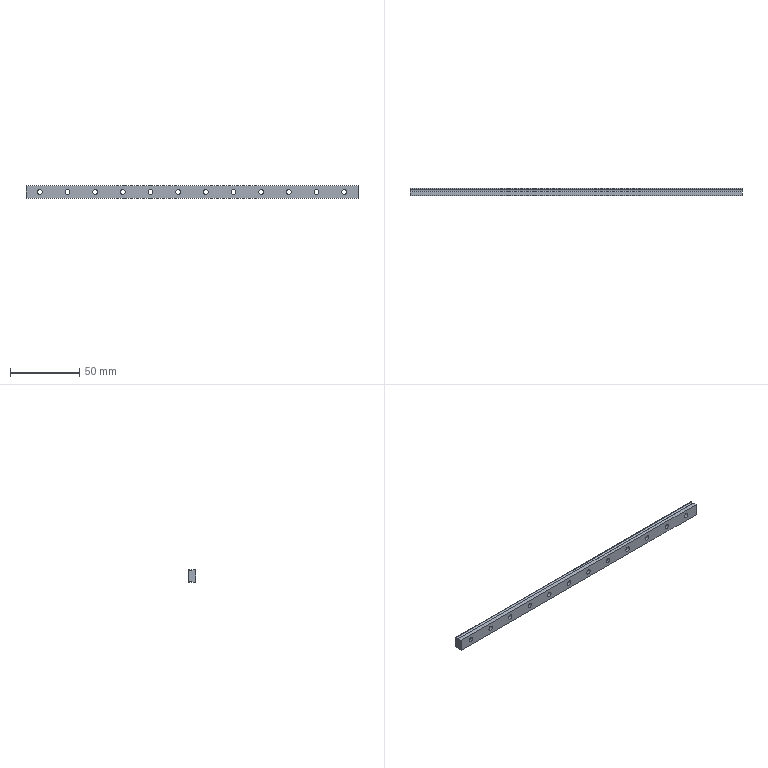Part | STEP file | RSR9KM1-250-1 | 1 solid | 48 faces | box 240 x 5.5 x 9 mm | volume 9857 mm3 | cylinder 26 | plane 22 | commonest cylinder face diameters 3.5 x12 6 x12 2 x2
STEP:
#1=CARTESIAN_POINT('',(230.,0.,4.5));
#2=VERTEX_POINT('',#1);
#3=CARTESIAN_POINT('',(230.,0.,-4.5));
#4=VERTEX_POINT('',#3);
#5=CARTESIAN_POINT('',(230.,0.,4.5));
#6=DIRECTION('',(0.,0.,-1.));
#7=VECTOR('',#6,1000.);
#8=LINE('',#5,#7);
#9=EDGE_CURVE('',#2,#4,#8,.T.);
#10=ORIENTED_EDGE('',*,*,#9,.F.);
#11=CARTESIAN_POINT('',(-10.,0.,4.5));
#12=VERTEX_POINT('',#11);
#13=CARTESIAN_POINT('',(-5.,0.,4.5));
#14=DIRECTION('',(-1.,0.,0.));
#15=VECTOR('',#14,1000.);
#16=LINE('',#13,#15);
#17=EDGE_CURVE('',#2,#12,#16,.T.);
#18=ORIENTED_EDGE('',*,*,#17,.T.);
#19=CARTESIAN_POINT('',(-10.,0.,-4.5));
#20=VERTEX_POINT('',#19);
#21=CARTESIAN_POINT('',(-10.,0.,-4.5));
#22=DIRECTION('',(0.,0.,1.));
#23=VECTOR('',#22,1000.);
#24=LINE('',#21,#23);
#25=EDGE_CURVE('',#20,#12,#24,.T.);
#26=ORIENTED_EDGE('',*,*,#25,.F.);
#27=CARTESIAN_POINT('',(-5.,0.,-4.5));
#28=DIRECTION('',(1.,0.,0.));
#29=VECTOR('',#28,1000.);
#30=LINE('',#27,#29);
#31=EDGE_CURVE('',#20,#4,#30,.T.);
#32=ORIENTED_EDGE('',*,*,#31,.T.);
#33=EDGE_LOOP('',(#10,#18,#26,#32));
#34=FACE_OUTER_BOUND('',#33,.T.);
#35=CARTESIAN_POINT('',(0.,0.,1.75));
#36=VERTEX_POINT('',#35);
#37=CARTESIAN_POINT('',(0.,0.,0.));
#38=DIRECTION('',(0.,1.,0.));
#39=DIRECTION('',(0.,0.,1.));
#40=AXIS2_PLACEMENT_3D('',#37,#38,#39);
#41=CIRCLE('',#40,1.75);
#42=EDGE_CURVE('',#36,#36,#41,.T.);
#43=ORIENTED_EDGE('',*,*,#42,.T.);
#44=EDGE_LOOP('',(#43));
#45=FACE_BOUND('',#44,.T.);
#46=CARTESIAN_POINT('',(220.,0.,1.75));
#47=VERTEX_POINT('',#46);
#48=CARTESIAN_POINT('',(220.,0.,0.));
#49=DIRECTION('',(0.,1.,0.));
#50=DIRECTION('',(0.,0.,1.));
#51=AXIS2_PLACEMENT_3D('',#48,#49,#50);
#52=CIRCLE('',#51,1.75);
#53=EDGE_CURVE('',#47,#47,#52,.T.);
#54=ORIENTED_EDGE('',*,*,#53,.T.);
#55=EDGE_LOOP('',(#54));
#56=FACE_BOUND('',#55,.T.);
#57=CARTESIAN_POINT('',(200.,0.,1.75));
#58=VERTEX_POINT('',#57);
#59=CARTESIAN_POINT('',(200.,0.,0.));
#60=DIRECTION('',(0.,1.,0.));
#61=DIRECTION('',(0.,0.,1.));
#62=AXIS2_PLACEMENT_3D('',#59,#60,#61);
#63=CIRCLE('',#62,1.75);
#64=EDGE_CURVE('',#58,#58,#63,.T.);
#65=ORIENTED_EDGE('',*,*,#64,.T.);
#66=EDGE_LOOP('',(#65));
#67=FACE_BOUND('',#66,.T.);
#68=CARTESIAN_POINT('',(180.,0.,1.75));
#69=VERTEX_POINT('',#68);
#70=CARTESIAN_POINT('',(180.,0.,0.));
#71=DIRECTION('',(0.,1.,0.));
#72=DIRECTION('',(0.,0.,1.));
#73=AXIS2_PLACEMENT_3D('',#70,#71,#72);
#74=CIRCLE('',#73,1.75);
#75=EDGE_CURVE('',#69,#69,#74,.T.);
#76=ORIENTED_EDGE('',*,*,#75,.T.);
#77=EDGE_LOOP('',(#76));
#78=FACE_BOUND('',#77,.T.);
#79=CARTESIAN_POINT('',(160.,0.,1.75));
#80=VERTEX_POINT('',#79);
#81=CARTESIAN_POINT('',(160.,0.,0.));
#82=DIRECTION('',(0.,1.,0.));
#83=DIRECTION('',(0.,0.,1.));
#84=AXIS2_PLACEMENT_3D('',#81,#82,#83);
#85=CIRCLE('',#84,1.75);
#86=EDGE_CURVE('',#80,#80,#85,.T.);
#87=ORIENTED_EDGE('',*,*,#86,.T.);
#88=EDGE_LOOP('',(#87));
#89=FACE_BOUND('',#88,.T.);
#90=CARTESIAN_POINT('',(140.,0.,1.75));
#91=VERTEX_POINT('',#90);
#92=CARTESIAN_POINT('',(140.,0.,0.));
#93=DIRECTION('',(0.,1.,0.));
#94=DIRECTION('',(0.,0.,1.));
#95=AXIS2_PLACEMENT_3D('',#92,#93,#94);
#96=CIRCLE('',#95,1.75);
#97=EDGE_CURVE('',#91,#91,#96,.T.);
#98=ORIENTED_EDGE('',*,*,#97,.T.);
#99=EDGE_LOOP('',(#98));
#100=FACE_BOUND('',#99,.T.);
#101=CARTESIAN_POINT('',(120.,0.,1.75));
#102=VERTEX_POINT('',#101);
#103=CARTESIAN_POINT('',(120.,0.,0.));
#104=DIRECTION('',(0.,1.,0.));
#105=DIRECTION('',(0.,0.,1.));
#106=AXIS2_PLACEMENT_3D('',#103,#104,#105);
#107=CIRCLE('',#106,1.75);
#108=EDGE_CURVE('',#102,#102,#107,.T.);
#109=ORIENTED_EDGE('',*,*,#108,.T.);
#110=EDGE_LOOP('',(#109));
#111=FACE_BOUND('',#110,.T.);
#112=CARTESIAN_POINT('',(100.,0.,1.75));
#113=VERTEX_POINT('',#112);
#114=CARTESIAN_POINT('',(100.,0.,0.));
#115=DIRECTION('',(0.,1.,0.));
#116=DIRECTION('',(0.,0.,1.));
#117=AXIS2_PLACEMENT_3D('',#114,#115,#116);
#118=CIRCLE('',#117,1.75);
#119=EDGE_CURVE('',#113,#113,#118,.T.);
#120=ORIENTED_EDGE('',*,*,#119,.T.);
#121=EDGE_LOOP('',(#120));
#122=FACE_BOUND('',#121,.T.);
#123=CARTESIAN_POINT('',(80.,0.,1.75));
#124=VERTEX_POINT('',#123);
#125=CARTESIAN_POINT('',(80.,0.,0.));
#126=DIRECTION('',(0.,1.,0.));
#127=DIRECTION('',(0.,0.,1.));
#128=AXIS2_PLACEMENT_3D('',#125,#126,#127);
#129=CIRCLE('',#128,1.75);
#130=EDGE_CURVE('',#124,#124,#129,.T.);
#131=ORIENTED_EDGE('',*,*,#130,.T.);
#132=EDGE_LOOP('',(#131));
#133=FACE_BOUND('',#132,.T.);
#134=CARTESIAN_POINT('',(60.,0.,1.75));
#135=VERTEX_POINT('',#134);
#136=CARTESIAN_POINT('',(60.,0.,0.));
#137=DIRECTION('',(0.,1.,0.));
#138=DIRECTION('',(0.,0.,1.));
#139=AXIS2_PLACEMENT_3D('',#136,#137,#138);
#140=CIRCLE('',#139,1.75);
#141=EDGE_CURVE('',#135,#135,#140,.T.);
#142=ORIENTED_EDGE('',*,*,#141,.T.);
#143=EDGE_LOOP('',(#142));
#144=FACE_BOUND('',#143,.T.);
#145=CARTESIAN_POINT('',(40.,0.,1.75));
#146=VERTEX_POINT('',#145);
#147=CARTESIAN_POINT('',(40.,0.,0.));
#148=DIRECTION('',(0.,1.,0.));
#149=DIRECTION('',(0.,0.,1.));
#150=AXIS2_PLACEMENT_3D('',#147,#148,#149);
#151=CIRCLE('',#150,1.75);
#152=EDGE_CURVE('',#146,#146,#151,.T.);
#153=ORIENTED_EDGE('',*,*,#152,.T.);
#154=EDGE_LOOP('',(#153));
#155=FACE_BOUND('',#154,.T.);
#156=CARTESIAN_POINT('',(20.,0.,1.75));
#157=VERTEX_POINT('',#156);
#158=CARTESIAN_POINT('',(20.,0.,0.));
#159=DIRECTION('',(0.,1.,0.));
#160=DIRECTION('',(0.,0.,1.));
#161=AXIS2_PLACEMENT_3D('',#158,#159,#160);
#162=CIRCLE('',#161,1.75);
#163=EDGE_CURVE('',#157,#157,#162,.T.);
#164=ORIENTED_EDGE('',*,*,#163,.T.);
#165=EDGE_LOOP('',(#164));
#166=FACE_BOUND('',#165,.T.);
#167=CARTESIAN_POINT('',(-5.,0.,-4.5));
#168=DIRECTION('',(0.,-1.,0.));
#169=DIRECTION('',(0.,0.,-1.));
#170=AXIS2_PLACEMENT_3D('',#167,#168,#169);
#171=PLANE('',#170);
#172=ADVANCED_FACE('',(#34,#45,#56,#67,#78,#89,#100,#111,#122,#133,#144,#155,#166),#171,.T.);
#173=CARTESIAN_POINT('',(230.,2.811,-4.5));
#174=VERTEX_POINT('',#173);
#175=CARTESIAN_POINT('',(230.,5.5,-4.5));
#176=DIRECTION('',(0.,-1.,0.));
#177=VECTOR('',#176,1000.);
#178=LINE('',#175,#177);
#179=EDGE_CURVE('',#174,#4,#178,.T.);
#180=ORIENTED_EDGE('',*,*,#179,.T.);
#181=ORIENTED_EDGE('',*,*,#31,.F.);
#182=CARTESIAN_POINT('',(-10.,2.811,-4.5));
#183=VERTEX_POINT('',#182);
#184=CARTESIAN_POINT('',(-10.,2.811,-4.5));
#185=DIRECTION('',(0.,-1.,0.));
#186=VECTOR('',#185,1000.);
#187=LINE('',#184,#186);
#188=EDGE_CURVE('',#183,#20,#187,.T.);
#189=ORIENTED_EDGE('',*,*,#188,.F.);
#190=CARTESIAN_POINT('',(-5.,2.811,-4.5));
#191=DIRECTION('',(1.,0.,0.));
#192=VECTOR('',#191,1000.);
#193=LINE('',#190,#192);
#194=EDGE_CURVE('',#183,#174,#193,.T.);
#195=ORIENTED_EDGE('',*,*,#194,.T.);
#196=EDGE_LOOP('',(#180,#181,#189,#195));
#197=FACE_OUTER_BOUND('',#196,.T.);
#198=CARTESIAN_POINT('',(-5.,2.811,-4.5));
#199=DIRECTION('',(0.,0.,-1.));
#200=DIRECTION('',(-1.,0.,0.));
#201=AXIS2_PLACEMENT_3D('',#198,#199,#200);
#202=PLANE('',#201);
#203=ADVANCED_FACE('',(#197),#202,.T.);
#204=CARTESIAN_POINT('',(230.,2.811,4.5));
#205=VERTEX_POINT('',#204);
#206=CARTESIAN_POINT('',(230.,5.5,4.5));
#207=DIRECTION('',(0.,-1.,0.));
#208=VECTOR('',#207,1000.);
#209=LINE('',#206,#208);
#210=EDGE_CURVE('',#205,#2,#209,.T.);
#211=ORIENTED_EDGE('',*,*,#210,.F.);
#212=CARTESIAN_POINT('',(-10.,2.811,4.5));
#213=VERTEX_POINT('',#212);
#214=CARTESIAN_POINT('',(-5.,2.811,4.5));
#215=DIRECTION('',(-1.,0.,0.));
#216=VECTOR('',#215,1000.);
#217=LINE('',#214,#216);
#218=EDGE_CURVE('',#205,#213,#217,.T.);
#219=ORIENTED_EDGE('',*,*,#218,.T.);
#220=CARTESIAN_POINT('',(-10.,0.,4.5));
#221=DIRECTION('',(0.,1.,0.));
#222=VECTOR('',#221,1000.);
#223=LINE('',#220,#222);
#224=EDGE_CURVE('',#12,#213,#223,.T.);
#225=ORIENTED_EDGE('',*,*,#224,.F.);
#226=ORIENTED_EDGE('',*,*,#17,.F.);
#227=EDGE_LOOP('',(#211,#219,#225,#226));
#228=FACE_OUTER_BOUND('',#227,.T.);
#229=CARTESIAN_POINT('',(-5.,0.,4.5));
#230=DIRECTION('',(0.,0.,1.));
#231=DIRECTION('',(1.,0.,0.));
#232=AXIS2_PLACEMENT_3D('',#229,#230,#231);
#233=PLANE('',#232);
#234=ADVANCED_FACE('',(#228),#233,.T.);
#235=ORIENTED_EDGE('',*,*,#42,.F.);
#236=EDGE_LOOP('',(#235));
#237=FACE_OUTER_BOUND('',#236,.T.);
#238=CARTESIAN_POINT('',(0.,2.2,1.75));
#239=VERTEX_POINT('',#238);
#240=CARTESIAN_POINT('',(0.,2.2,0.));
#241=DIRECTION('',(0.,-1.,0.));
#242=DIRECTION('',(0.,0.,1.));
#243=AXIS2_PLACEMENT_3D('',#240,#241,#242);
#244=CIRCLE('',#243,1.75);
#245=EDGE_CURVE('',#239,#239,#244,.T.);
#246=ORIENTED_EDGE('',*,*,#245,.F.);
#247=EDGE_LOOP('',(#246));
#248=FACE_OUTER_BOUND('',#247,.T.);
#249=CARTESIAN_POINT('',(0.,1.1,0.));
#250=DIRECTION('',(0.,1.,0.));
#251=DIRECTION('',(0.,0.,1.));
#252=AXIS2_PLACEMENT_3D('',#249,#250,#251);
#253=CYLINDRICAL_SURFACE('',#252,1.75);
#254=ADVANCED_FACE('',(#237,#248),#253,.F.);
#255=ORIENTED_EDGE('',*,*,#53,.F.);
#256=EDGE_LOOP('',(#255));
#257=FACE_OUTER_BOUND('',#256,.T.);
#258=CARTESIAN_POINT('',(220.,2.2,1.75));
#259=VERTEX_POINT('',#258);
#260=CARTESIAN_POINT('',(220.,2.2,0.));
#261=DIRECTION('',(0.,-1.,0.));
#262=DIRECTION('',(0.,0.,1.));
#263=AXIS2_PLACEMENT_3D('',#260,#261,#262);
#264=CIRCLE('',#263,1.75);
#265=EDGE_CURVE('',#259,#259,#264,.T.);
#266=ORIENTED_EDGE('',*,*,#265,.F.);
#267=EDGE_LOOP('',(#266));
#268=FACE_OUTER_BOUND('',#267,.T.);
#269=CARTESIAN_POINT('',(220.,1.1,0.));
#270=DIRECTION('',(0.,1.,0.));
#271=DIRECTION('',(0.,0.,1.));
#272=AXIS2_PLACEMENT_3D('',#269,#270,#271);
#273=CYLINDRICAL_SURFACE('',#272,1.75);
#274=ADVANCED_FACE('',(#257,#268),#273,.F.);
#275=ORIENTED_EDGE('',*,*,#64,.F.);
#276=EDGE_LOOP('',(#275));
#277=FACE_OUTER_BOUND('',#276,.T.);
#278=CARTESIAN_POINT('',(200.,2.2,1.75));
#279=VERTEX_POINT('',#278);
#280=CARTESIAN_POINT('',(200.,2.2,0.));
#281=DIRECTION('',(0.,-1.,0.));
#282=DIRECTION('',(0.,0.,1.));
#283=AXIS2_PLACEMENT_3D('',#280,#281,#282);
#284=CIRCLE('',#283,1.75);
#285=EDGE_CURVE('',#279,#279,#284,.T.);
#286=ORIENTED_EDGE('',*,*,#285,.F.);
#287=EDGE_LOOP('',(#286));
#288=FACE_OUTER_BOUND('',#287,.T.);
#289=CARTESIAN_POINT('',(200.,1.1,0.));
#290=DIRECTION('',(0.,1.,0.));
#291=DIRECTION('',(0.,0.,1.));
#292=AXIS2_PLACEMENT_3D('',#289,#290,#291);
#293=CYLINDRICAL_SURFACE('',#292,1.75);
#294=ADVANCED_FACE('',(#277,#288),#293,.F.);
#295=ORIENTED_EDGE('',*,*,#75,.F.);
#296=EDGE_LOOP('',(#295));
#297=FACE_OUTER_BOUND('',#296,.T.);
#298=CARTESIAN_POINT('',(180.,2.2,1.75));
#299=VERTEX_POINT('',#298);
#300=CARTESIAN_POINT('',(180.,2.2,0.));
#301=DIRECTION('',(0.,-1.,0.));
#302=DIRECTION('',(0.,0.,1.));
#303=AXIS2_PLACEMENT_3D('',#300,#301,#302);
#304=CIRCLE('',#303,1.75);
#305=EDGE_CURVE('',#299,#299,#304,.T.);
#306=ORIENTED_EDGE('',*,*,#305,.F.);
#307=EDGE_LOOP('',(#306));
#308=FACE_OUTER_BOUND('',#307,.T.);
#309=CARTESIAN_POINT('',(180.,1.1,0.));
#310=DIRECTION('',(0.,1.,0.));
#311=DIRECTION('',(0.,0.,1.));
#312=AXIS2_PLACEMENT_3D('',#309,#310,#311);
#313=CYLINDRICAL_SURFACE('',#312,1.75);
#314=ADVANCED_FACE('',(#297,#308),#313,.F.);
#315=ORIENTED_EDGE('',*,*,#86,.F.);
#316=EDGE_LOOP('',(#315));
#317=FACE_OUTER_BOUND('',#316,.T.);
#318=CARTESIAN_POINT('',(160.,2.2,1.75));
#319=VERTEX_POINT('',#318);
#320=CARTESIAN_POINT('',(160.,2.2,0.));
#321=DIRECTION('',(0.,-1.,0.));
#322=DIRECTION('',(0.,0.,1.));
#323=AXIS2_PLACEMENT_3D('',#320,#321,#322);
#324=CIRCLE('',#323,1.75);
#325=EDGE_CURVE('',#319,#319,#324,.T.);
#326=ORIENTED_EDGE('',*,*,#325,.F.);
#327=EDGE_LOOP('',(#326));
#328=FACE_OUTER_BOUND('',#327,.T.);
#329=CARTESIAN_POINT('',(160.,1.1,0.));
#330=DIRECTION('',(0.,1.,0.));
#331=DIRECTION('',(0.,0.,1.));
#332=AXIS2_PLACEMENT_3D('',#329,#330,#331);
#333=CYLINDRICAL_SURFACE('',#332,1.75);
#334=ADVANCED_FACE('',(#317,#328),#333,.F.);
#335=ORIENTED_EDGE('',*,*,#97,.F.);
#336=EDGE_LOOP('',(#335));
#337=FACE_OUTER_BOUND('',#336,.T.);
#338=CARTESIAN_POINT('',(140.,2.2,1.75));
#339=VERTEX_POINT('',#338);
#340=CARTESIAN_POINT('',(140.,2.2,0.));
#341=DIRECTION('',(0.,-1.,0.));
#342=DIRECTION('',(0.,0.,1.));
#343=AXIS2_PLACEMENT_3D('',#340,#341,#342);
#344=CIRCLE('',#343,1.75);
#345=EDGE_CURVE('',#339,#339,#344,.T.);
#346=ORIENTED_EDGE('',*,*,#345,.F.);
#347=EDGE_LOOP('',(#346));
#348=FACE_OUTER_BOUND('',#347,.T.);
#349=CARTESIAN_POINT('',(140.,1.1,0.));
#350=DIRECTION('',(0.,1.,0.));
#351=DIRECTION('',(0.,0.,1.));
#352=AXIS2_PLACEMENT_3D('',#349,#350,#351);
#353=CYLINDRICAL_SURFACE('',#352,1.75);
#354=ADVANCED_FACE('',(#337,#348),#353,.F.);
#355=ORIENTED_EDGE('',*,*,#108,.F.);
#356=EDGE_LOOP('',(#355));
#357=FACE_OUTER_BOUND('',#356,.T.);
#358=CARTESIAN_POINT('',(120.,2.2,1.75));
#359=VERTEX_POINT('',#358);
#360=CARTESIAN_POINT('',(120.,2.2,0.));
#361=DIRECTION('',(0.,-1.,0.));
#362=DIRECTION('',(0.,0.,1.));
#363=AXIS2_PLACEMENT_3D('',#360,#361,#362);
#364=CIRCLE('',#363,1.75);
#365=EDGE_CURVE('',#359,#359,#364,.T.);
#366=ORIENTED_EDGE('',*,*,#365,.F.);
#367=EDGE_LOOP('',(#366));
#368=FACE_OUTER_BOUND('',#367,.T.);
#369=CARTESIAN_POINT('',(120.,1.1,0.));
#370=DIRECTION('',(0.,1.,0.));
#371=DIRECTION('',(0.,0.,1.));
#372=AXIS2_PLACEMENT_3D('',#369,#370,#371);
#373=CYLINDRICAL_SURFACE('',#372,1.75);
#374=ADVANCED_FACE('',(#357,#368),#373,.F.);
#375=ORIENTED_EDGE('',*,*,#119,.F.);
#376=EDGE_LOOP('',(#375));
#377=FACE_OUTER_BOUND('',#376,.T.);
#378=CARTESIAN_POINT('',(100.,2.2,1.75));
#379=VERTEX_POINT('',#378);
#380=CARTESIAN_POINT('',(100.,2.2,0.));
#381=DIRECTION('',(0.,-1.,0.));
#382=DIRECTION('',(0.,0.,1.));
#383=AXIS2_PLACEMENT_3D('',#380,#381,#382);
#384=CIRCLE('',#383,1.75);
#385=EDGE_CURVE('',#379,#379,#384,.T.);
#386=ORIENTED_EDGE('',*,*,#385,.F.);
#387=EDGE_LOOP('',(#386));
#388=FACE_OUTER_BOUND('',#387,.T.);
#389=CARTESIAN_POINT('',(100.,1.1,0.));
#390=DIRECTION('',(0.,1.,0.));
#391=DIRECTION('',(0.,0.,1.));
#392=AXIS2_PLACEMENT_3D('',#389,#390,#391);
#393=CYLINDRICAL_SURFACE('',#392,1.75);
#394=ADVANCED_FACE('',(#377,#388),#393,.F.);
#395=ORIENTED_EDGE('',*,*,#130,.F.);
#396=EDGE_LOOP('',(#395));
#397=FACE_OUTER_BOUND('',#396,.T.);
#398=CARTESIAN_POINT('',(80.,2.2,1.75));
#399=VERTEX_POINT('',#398);
#400=CARTESIAN_POINT('',(80.,2.2,0.));
#401=DIRECTION('',(0.,-1.,0.));
#402=DIRECTION('',(0.,0.,1.));
#403=AXIS2_PLACEMENT_3D('',#400,#401,#402);
#404=CIRCLE('',#403,1.75);
#405=EDGE_CURVE('',#399,#399,#404,.T.);
#406=ORIENTED_EDGE('',*,*,#405,.F.);
#407=EDGE_LOOP('',(#406));
#408=FACE_OUTER_BOUND('',#407,.T.);
#409=CARTESIAN_POINT('',(80.,1.1,0.));
#410=DIRECTION('',(0.,1.,0.));
#411=DIRECTION('',(0.,0.,1.));
#412=AXIS2_PLACEMENT_3D('',#409,#410,#411);
#413=CYLINDRICAL_SURFACE('',#412,1.75);
#414=ADVANCED_FACE('',(#397,#408),#413,.F.);
#415=ORIENTED_EDGE('',*,*,#141,.F.);
#416=EDGE_LOOP('',(#415));
#417=FACE_OUTER_BOUND('',#416,.T.);
#418=CARTESIAN_POINT('',(60.,2.2,1.75));
#419=VERTEX_POINT('',#418);
#420=CARTESIAN_POINT('',(60.,2.2,0.));
#421=DIRECTION('',(0.,-1.,0.));
#422=DIRECTION('',(0.,0.,1.));
#423=AXIS2_PLACEMENT_3D('',#420,#421,#422);
#424=CIRCLE('',#423,1.75);
#425=EDGE_CURVE('',#419,#419,#424,.T.);
#426=ORIENTED_EDGE('',*,*,#425,.F.);
#427=EDGE_LOOP('',(#426));
#428=FACE_OUTER_BOUND('',#427,.T.);
#429=CARTESIAN_POINT('',(60.,1.1,0.));
#430=DIRECTION('',(0.,1.,0.));
#431=DIRECTION('',(0.,0.,1.));
#432=AXIS2_PLACEMENT_3D('',#429,#430,#431);
#433=CYLINDRICAL_SURFACE('',#432,1.75);
#434=ADVANCED_FACE('',(#417,#428),#433,.F.);
#435=ORIENTED_EDGE('',*,*,#152,.F.);
#436=EDGE_LOOP('',(#435));
#437=FACE_OUTER_BOUND('',#436,.T.);
#438=CARTESIAN_POINT('',(40.,2.2,1.75));
#439=VERTEX_POINT('',#438);
#440=CARTESIAN_POINT('',(40.,2.2,0.));
#441=DIRECTION('',(0.,-1.,0.));
#442=DIRECTION('',(0.,0.,1.));
#443=AXIS2_PLACEMENT_3D('',#440,#441,#442);
#444=CIRCLE('',#443,1.75);
#445=EDGE_CURVE('',#439,#439,#444,.T.);
#446=ORIENTED_EDGE('',*,*,#445,.F.);
#447=EDGE_LOOP('',(#446));
#448=FACE_OUTER_BOUND('',#447,.T.);
#449=CARTESIAN_POINT('',(40.,1.1,0.));
#450=DIRECTION('',(0.,1.,0.));
#451=DIRECTION('',(0.,0.,1.));
#452=AXIS2_PLACEMENT_3D('',#449,#450,#451);
#453=CYLINDRICAL_SURFACE('',#452,1.75);
#454=ADVANCED_FACE('',(#437,#448),#453,.F.);
#455=ORIENTED_EDGE('',*,*,#163,.F.);
#456=EDGE_LOOP('',(#455));
#457=FACE_OUTER_BOUND('',#456,.T.);
#458=CARTESIAN_POINT('',(20.,2.2,1.75));
#459=VERTEX_POINT('',#458);
#460=CARTESIAN_POINT('',(20.,2.2,0.));
#461=DIRECTION('',(0.,-1.,0.));
#462=DIRECTION('',(0.,0.,1.));
#463=AXIS2_PLACEMENT_3D('',#460,#461,#462);
#464=CIRCLE('',#463,1.75);
#465=EDGE_CURVE('',#459,#459,#464,.T.);
#466=ORIENTED_EDGE('',*,*,#465,.F.);
#467=EDGE_LOOP('',(#466));
#468=FACE_OUTER_BOUND('',#467,.T.);
#469=CARTESIAN_POINT('',(20.,1.1,0.));
#470=DIRECTION('',(0.,1.,0.));
#471=DIRECTION('',(0.,0.,1.));
#472=AXIS2_PLACEMENT_3D('',#469,#470,#471);
#473=CYLINDRICAL_SURFACE('',#472,1.75);
#474=ADVANCED_FACE('',(#457,#468),#473,.F.);
#475=CARTESIAN_POINT('',(230.,4.789,-4.5));
#476=VERTEX_POINT('',#475);
#477=CARTESIAN_POINT('',(230.,3.8,-4.65));
#478=DIRECTION('',(-1.,0.,0.));
#479=DIRECTION('',(0.,0.,1.));
#480=AXIS2_PLACEMENT_3D('',#477,#478,#479);
#481=CIRCLE('',#480,1.);
#482=EDGE_CURVE('',#174,#476,#481,.T.);
#483=ORIENTED_EDGE('',*,*,#482,.F.);
#484=ORIENTED_EDGE('',*,*,#194,.F.);
#485=CARTESIAN_POINT('',(-10.,4.789,-4.5));
#486=VERTEX_POINT('',#485);
#487=CARTESIAN_POINT('',(-10.,3.8,-4.65));
#488=DIRECTION('',(1.,0.,0.));
#489=DIRECTION('',(0.,0.,1.));
#490=AXIS2_PLACEMENT_3D('',#487,#488,#489);
#491=CIRCLE('',#490,1.);
#492=EDGE_CURVE('',#486,#183,#491,.T.);
#493=ORIENTED_EDGE('',*,*,#492,.F.);
#494=CARTESIAN_POINT('',(-5.,4.789,-4.5));
#495=DIRECTION('',(1.,0.,0.));
#496=VECTOR('',#495,1000.);
#497=LINE('',#494,#496);
#498=EDGE_CURVE('',#486,#476,#497,.T.);
#499=ORIENTED_EDGE('',*,*,#498,.T.);
#500=EDGE_LOOP('',(#483,#484,#493,#499));
#501=FACE_OUTER_BOUND('',#500,.T.);
#502=CARTESIAN_POINT('',(-5.,3.8,-4.65));
#503=DIRECTION('',(1.,0.,0.));
#504=DIRECTION('',(0.,0.,-1.));
#505=AXIS2_PLACEMENT_3D('',#502,#503,#504);
#506=CYLINDRICAL_SURFACE('',#505,1.);
#507=ADVANCED_FACE('',(#501),#506,.F.);
#508=CARTESIAN_POINT('',(230.,4.789,4.5));
#509=VERTEX_POINT('',#508);
#510=CARTESIAN_POINT('',(230.,3.8,4.65));
#511=DIRECTION('',(-1.,0.,0.));
#512=DIRECTION('',(0.,0.,1.));
#513=AXIS2_PLACEMENT_3D('',#510,#511,#512);
#514=CIRCLE('',#513,1.);
#515=EDGE_CURVE('',#509,#205,#514,.T.);
#516=ORIENTED_EDGE('',*,*,#515,.F.);
#517=CARTESIAN_POINT('',(-10.,4.789,4.5));
#518=VERTEX_POINT('',#517);
#519=CARTESIAN_POINT('',(-5.,4.789,4.5));
#520=DIRECTION('',(-1.,0.,0.));
#521=VECTOR('',#520,1000.);
#522=LINE('',#519,#521);
#523=EDGE_CURVE('',#509,#518,#522,.T.);
#524=ORIENTED_EDGE('',*,*,#523,.T.);
#525=CARTESIAN_POINT('',(-10.,3.8,4.65));
#526=DIRECTION('',(1.,0.,0.));
#527=DIRECTION('',(0.,0.,1.));
#528=AXIS2_PLACEMENT_3D('',#525,#526,#527);
#529=CIRCLE('',#528,1.);
#530=EDGE_CURVE('',#213,#518,#529,.T.);
#531=ORIENTED_EDGE('',*,*,#530,.F.);
#532=ORIENTED_EDGE('',*,*,#218,.F.);
#533=EDGE_LOOP('',(#516,#524,#531,#532));
#534=FACE_OUTER_BOUND('',#533,.T.);
#535=CARTESIAN_POINT('',(-5.,3.8,4.65));
#536=DIRECTION('',(1.,0.,0.));
#537=DIRECTION('',(0.,0.,-1.));
#538=AXIS2_PLACEMENT_3D('',#535,#536,#537);
#539=CYLINDRICAL_SURFACE('',#538,1.);
#540=ADVANCED_FACE('',(#534),#539,.F.);
#541=CARTESIAN_POINT('',(230.,5.5,4.1));
#542=VERTEX_POINT('',#541);
#543=CARTESIAN_POINT('',(230.,5.5,-4.1));
#544=VERTEX_POINT('',#543);
#545=CARTESIAN_POINT('',(230.,5.5,4.5));
#546=DIRECTION('',(0.,0.,-1.));
#547=VECTOR('',#546,1000.);
#548=LINE('',#545,#547);
#549=EDGE_CURVE('',#542,#544,#548,.T.);
#550=ORIENTED_EDGE('',*,*,#549,.T.);
#551=CARTESIAN_POINT('',(-10.,5.5,-4.1));
#552=VERTEX_POINT('',#551);
#553=CARTESIAN_POINT('',(-5.,5.5,-4.1));
#554=DIRECTION('',(-1.,0.,0.));
#555=VECTOR('',#554,1000.);
#556=LINE('',#553,#555);
#557=EDGE_CURVE('',#544,#552,#556,.T.);
#558=ORIENTED_EDGE('',*,*,#557,.T.);
#559=CARTESIAN_POINT('',(-10.,5.5,4.1));
#560=VERTEX_POINT('',#559);
#561=CARTESIAN_POINT('',(-10.,5.5,4.1));
#562=DIRECTION('',(0.,0.,-1.));
#563=VECTOR('',#562,1000.);
#564=LINE('',#561,#563);
#565=EDGE_CURVE('',#560,#552,#564,.T.);
#566=ORIENTED_EDGE('',*,*,#565,.F.);
#567=CARTESIAN_POINT('',(-5.,5.5,4.1));
#568=DIRECTION('',(1.,0.,0.));
#569=VECTOR('',#568,1000.);
#570=LINE('',#567,#569);
#571=EDGE_CURVE('',#560,#542,#570,.T.);
#572=ORIENTED_EDGE('',*,*,#571,.T.);
#573=EDGE_LOOP('',(#550,#558,#566,#572));
#574=FACE_OUTER_BOUND('',#573,.T.);
#575=CARTESIAN_POINT('',(0.,5.5,3.));
#576=VERTEX_POINT('',#575);
#577=CARTESIAN_POINT('',(0.,5.5,0.));
#578=DIRECTION('',(0.,-1.,0.));
#579=DIRECTION('',(0.,0.,1.));
#580=AXIS2_PLACEMENT_3D('',#577,#578,#579);
#581=CIRCLE('',#580,3.);
#582=EDGE_CURVE('',#576,#576,#581,.T.);
#583=ORIENTED_EDGE('',*,*,#582,.T.);
#584=EDGE_LOOP('',(#583));
#585=FACE_BOUND('',#584,.T.);
#586=CARTESIAN_POINT('',(220.,5.5,3.));
#587=VERTEX_POINT('',#586);
#588=CARTESIAN_POINT('',(220.,5.5,0.));
#589=DIRECTION('',(0.,-1.,0.));
#590=DIRECTION('',(0.,0.,1.));
#591=AXIS2_PLACEMENT_3D('',#588,#589,#590);
#592=CIRCLE('',#591,3.);
#593=EDGE_CURVE('',#587,#587,#592,.T.);
#594=ORIENTED_EDGE('',*,*,#593,.T.);
#595=EDGE_LOOP('',(#594));
#596=FACE_BOUND('',#595,.T.);
#597=CARTESIAN_POINT('',(200.,5.5,3.));
#598=VERTEX_POINT('',#597);
#599=CARTESIAN_POINT('',(200.,5.5,0.));
#600=DIRECTION('',(0.,-1.,0.));
#601=DIRECTION('',(0.,0.,1.));
#602=AXIS2_PLACEMENT_3D('',#599,#600,#601);
#603=CIRCLE('',#602,3.);
#604=EDGE_CURVE('',#598,#598,#603,.T.);
#605=ORIENTED_EDGE('',*,*,#604,.T.);
#606=EDGE_LOOP('',(#605));
#607=FACE_BOUND('',#606,.T.);
#608=CARTESIAN_POINT('',(180.,5.5,3.));
#609=VERTEX_POINT('',#608);
#610=CARTESIAN_POINT('',(180.,5.5,0.));
#611=DIRECTION('',(0.,-1.,0.));
#612=DIRECTION('',(0.,0.,1.));
#613=AXIS2_PLACEMENT_3D('',#610,#611,#612);
#614=CIRCLE('',#613,3.);
#615=EDGE_CURVE('',#609,#609,#614,.T.);
#616=ORIENTED_EDGE('',*,*,#615,.T.);
#617=EDGE_LOOP('',(#616));
#618=FACE_BOUND('',#617,.T.);
#619=CARTESIAN_POINT('',(160.,5.5,3.));
#620=VERTEX_POINT('',#619);
#621=CARTESIAN_POINT('',(160.,5.5,0.));
#622=DIRECTION('',(0.,-1.,0.));
#623=DIRECTION('',(0.,0.,1.));
#624=AXIS2_PLACEMENT_3D('',#621,#622,#623);
#625=CIRCLE('',#624,3.);
#626=EDGE_CURVE('',#620,#620,#625,.T.);
#627=ORIENTED_EDGE('',*,*,#626,.T.);
#628=EDGE_LOOP('',(#627));
#629=FACE_BOUND('',#628,.T.);
#630=CARTESIAN_POINT('',(140.,5.5,3.));
#631=VERTEX_POINT('',#630);
#632=CARTESIAN_POINT('',(140.,5.5,0.));
#633=DIRECTION('',(0.,-1.,0.));
#634=DIRECTION('',(0.,0.,1.));
#635=AXIS2_PLACEMENT_3D('',#632,#633,#634);
#636=CIRCLE('',#635,3.);
#637=EDGE_CURVE('',#631,#631,#636,.T.);
#638=ORIENTED_EDGE('',*,*,#637,.T.);
#639=EDGE_LOOP('',(#638));
#640=FACE_BOUND('',#639,.T.);
#641=CARTESIAN_POINT('',(120.,5.5,3.));
#642=VERTEX_POINT('',#641);
#643=CARTESIAN_POINT('',(120.,5.5,0.));
#644=DIRECTION('',(0.,-1.,0.));
#645=DIRECTION('',(0.,0.,1.));
#646=AXIS2_PLACEMENT_3D('',#643,#644,#645);
#647=CIRCLE('',#646,3.);
#648=EDGE_CURVE('',#642,#642,#647,.T.);
#649=ORIENTED_EDGE('',*,*,#648,.T.);
#650=EDGE_LOOP('',(#649));
#651=FACE_BOUND('',#650,.T.);
#652=CARTESIAN_POINT('',(100.,5.5,3.));
#653=VERTEX_POINT('',#652);
#654=CARTESIAN_POINT('',(100.,5.5,0.));
#655=DIRECTION('',(0.,-1.,0.));
#656=DIRECTION('',(0.,0.,1.));
#657=AXIS2_PLACEMENT_3D('',#654,#655,#656);
#658=CIRCLE('',#657,3.);
#659=EDGE_CURVE('',#653,#653,#658,.T.);
#660=ORIENTED_EDGE('',*,*,#659,.T.);
#661=EDGE_LOOP('',(#660));
#662=FACE_BOUND('',#661,.T.);
#663=CARTESIAN_POINT('',(80.,5.5,3.));
#664=VERTEX_POINT('',#663);
#665=CARTESIAN_POINT('',(80.,5.5,0.));
#666=DIRECTION('',(0.,-1.,0.));
#667=DIRECTION('',(0.,0.,1.));
#668=AXIS2_PLACEMENT_3D('',#665,#666,#667);
#669=CIRCLE('',#668,3.);
#670=EDGE_CURVE('',#664,#664,#669,.T.);
#671=ORIENTED_EDGE('',*,*,#670,.T.);
#672=EDGE_LOOP('',(#671));
#673=FACE_BOUND('',#672,.T.);
#674=CARTESIAN_POINT('',(60.,5.5,3.));
#675=VERTEX_POINT('',#674);
#676=CARTESIAN_POINT('',(60.,5.5,0.));
#677=DIRECTION('',(0.,-1.,0.));
#678=DIRECTION('',(0.,0.,1.));
#679=AXIS2_PLACEMENT_3D('',#676,#677,#678);
#680=CIRCLE('',#679,3.);
#681=EDGE_CURVE('',#675,#675,#680,.T.);
#682=ORIENTED_EDGE('',*,*,#681,.T.);
#683=EDGE_LOOP('',(#682));
#684=FACE_BOUND('',#683,.T.);
#685=CARTESIAN_POINT('',(40.,5.5,3.));
#686=VERTEX_POINT('',#685);
#687=CARTESIAN_POINT('',(40.,5.5,0.));
#688=DIRECTION('',(0.,-1.,0.));
#689=DIRECTION('',(0.,0.,1.));
#690=AXIS2_PLACEMENT_3D('',#687,#688,#689);
#691=CIRCLE('',#690,3.);
#692=EDGE_CURVE('',#686,#686,#691,.T.);
#693=ORIENTED_EDGE('',*,*,#692,.T.);
#694=EDGE_LOOP('',(#693));
#695=FACE_BOUND('',#694,.T.);
#696=CARTESIAN_POINT('',(20.,5.5,3.));
#697=VERTEX_POINT('',#696);
#698=CARTESIAN_POINT('',(20.,5.5,0.));
#699=DIRECTION('',(0.,-1.,0.));
#700=DIRECTION('',(0.,0.,1.));
#701=AXIS2_PLACEMENT_3D('',#698,#699,#700);
#702=CIRCLE('',#701,3.);
#703=EDGE_CURVE('',#697,#697,#702,.T.);
#704=ORIENTED_EDGE('',*,*,#703,.T.);
#705=EDGE_LOOP('',(#704));
#706=FACE_BOUND('',#705,.T.);
#707=CARTESIAN_POINT('',(-5.,5.5,4.1));
#708=DIRECTION('',(0.,1.,0.));
#709=DIRECTION('',(0.,0.,1.));
#710=AXIS2_PLACEMENT_3D('',#707,#708,#709);
#711=PLANE('',#710);
#712=ADVANCED_FACE('',(#574,#585,#596,#607,#618,#629,#640,#651,#662,#673,#684,#695,#706),#711,.T.);
#713=ORIENTED_EDGE('',*,*,#245,.T.);
#714=EDGE_LOOP('',(#713));
#715=FACE_BOUND('',#714,.T.);
#716=CARTESIAN_POINT('',(0.,2.2,3.));
#717=VERTEX_POINT('',#716);
#718=CARTESIAN_POINT('',(0.,2.2,0.));
#719=DIRECTION('',(0.,-1.,0.));
#720=DIRECTION('',(0.,0.,1.));
#721=AXIS2_PLACEMENT_3D('',#718,#719,#720);
#722=CIRCLE('',#721,3.);
#723=EDGE_CURVE('',#717,#717,#722,.T.);
#724=ORIENTED_EDGE('',*,*,#723,.F.);
#725=EDGE_LOOP('',(#724));
#726=FACE_OUTER_BOUND('',#725,.T.);
#727=CARTESIAN_POINT('',(2.375,2.2,0.));
#728=DIRECTION('',(0.,-1.,0.));
#729=DIRECTION('',(1.,0.,0.));
#730=AXIS2_PLACEMENT_3D('',#727,#728,#729);
#731=PLANE('',#730);
#732=ADVANCED_FACE('',(#715,#726),#731,.F.);
#733=ORIENTED_EDGE('',*,*,#265,.T.);
#734=EDGE_LOOP('',(#733));
#735=FACE_BOUND('',#734,.T.);
#736=CARTESIAN_POINT('',(220.,2.2,3.));
#737=VERTEX_POINT('',#736);
#738=CARTESIAN_POINT('',(220.,2.2,0.));
#739=DIRECTION('',(0.,-1.,0.));
#740=DIRECTION('',(0.,0.,1.));
#741=AXIS2_PLACEMENT_3D('',#738,#739,#740);
#742=CIRCLE('',#741,3.);
#743=EDGE_CURVE('',#737,#737,#742,.T.);
#744=ORIENTED_EDGE('',*,*,#743,.F.);
#745=EDGE_LOOP('',(#744));
#746=FACE_OUTER_BOUND('',#745,.T.);
#747=CARTESIAN_POINT('',(222.375,2.2,0.));
#748=DIRECTION('',(0.,-1.,0.));
#749=DIRECTION('',(1.,0.,0.));
#750=AXIS2_PLACEMENT_3D('',#747,#748,#749);
#751=PLANE('',#750);
#752=ADVANCED_FACE('',(#735,#746),#751,.F.);
#753=ORIENTED_EDGE('',*,*,#285,.T.);
#754=EDGE_LOOP('',(#753));
#755=FACE_BOUND('',#754,.T.);
#756=CARTESIAN_POINT('',(200.,2.2,3.));
#757=VERTEX_POINT('',#756);
#758=CARTESIAN_POINT('',(200.,2.2,0.));
#759=DIRECTION('',(0.,-1.,0.));
#760=DIRECTION('',(0.,0.,1.));
#761=AXIS2_PLACEMENT_3D('',#758,#759,#760);
#762=CIRCLE('',#761,3.);
#763=EDGE_CURVE('',#757,#757,#762,.T.);
#764=ORIENTED_EDGE('',*,*,#763,.F.);
#765=EDGE_LOOP('',(#764));
#766=FACE_OUTER_BOUND('',#765,.T.);
#767=CARTESIAN_POINT('',(202.375,2.2,0.));
#768=DIRECTION('',(0.,-1.,0.));
#769=DIRECTION('',(1.,0.,0.));
#770=AXIS2_PLACEMENT_3D('',#767,#768,#769);
#771=PLANE('',#770);
#772=ADVANCED_FACE('',(#755,#766),#771,.F.);
#773=ORIENTED_EDGE('',*,*,#305,.T.);
#774=EDGE_LOOP('',(#773));
#775=FACE_BOUND('',#774,.T.);
#776=CARTESIAN_POINT('',(180.,2.2,3.));
#777=VERTEX_POINT('',#776);
#778=CARTESIAN_POINT('',(180.,2.2,0.));
#779=DIRECTION('',(0.,-1.,0.));
#780=DIRECTION('',(0.,0.,1.));
#781=AXIS2_PLACEMENT_3D('',#778,#779,#780);
#782=CIRCLE('',#781,3.);
#783=EDGE_CURVE('',#777,#777,#782,.T.);
#784=ORIENTED_EDGE('',*,*,#783,.F.);
#785=EDGE_LOOP('',(#784));
#786=FACE_OUTER_BOUND('',#785,.T.);
#787=CARTESIAN_POINT('',(182.375,2.2,0.));
#788=DIRECTION('',(0.,-1.,0.));
#789=DIRECTION('',(1.,0.,0.));
#790=AXIS2_PLACEMENT_3D('',#787,#788,#789);
#791=PLANE('',#790);
#792=ADVANCED_FACE('',(#775,#786),#791,.F.);
#793=ORIENTED_EDGE('',*,*,#325,.T.);
#794=EDGE_LOOP('',(#793));
#795=FACE_BOUND('',#794,.T.);
#796=CARTESIAN_POINT('',(160.,2.2,3.));
#797=VERTEX_POINT('',#796);
#798=CARTESIAN_POINT('',(160.,2.2,0.));
#799=DIRECTION('',(0.,-1.,0.));
#800=DIRECTION('',(0.,0.,1.));
#801=AXIS2_PLACEMENT_3D('',#798,#799,#800);
#802=CIRCLE('',#801,3.);
#803=EDGE_CURVE('',#797,#797,#802,.T.);
#804=ORIENTED_EDGE('',*,*,#803,.F.);
#805=EDGE_LOOP('',(#804));
#806=FACE_OUTER_BOUND('',#805,.T.);
#807=CARTESIAN_POINT('',(162.375,2.2,0.));
#808=DIRECTION('',(0.,-1.,0.));
#809=DIRECTION('',(1.,0.,0.));
#810=AXIS2_PLACEMENT_3D('',#807,#808,#809);
#811=PLANE('',#810);
#812=ADVANCED_FACE('',(#795,#806),#811,.F.);
#813=ORIENTED_EDGE('',*,*,#345,.T.);
#814=EDGE_LOOP('',(#813));
#815=FACE_BOUND('',#814,.T.);
#816=CARTESIAN_POINT('',(140.,2.2,3.));
#817=VERTEX_POINT('',#816);
#818=CARTESIAN_POINT('',(140.,2.2,0.));
#819=DIRECTION('',(0.,-1.,0.));
#820=DIRECTION('',(0.,0.,1.));
#821=AXIS2_PLACEMENT_3D('',#818,#819,#820);
#822=CIRCLE('',#821,3.);
#823=EDGE_CURVE('',#817,#817,#822,.T.);
#824=ORIENTED_EDGE('',*,*,#823,.F.);
#825=EDGE_LOOP('',(#824));
#826=FACE_OUTER_BOUND('',#825,.T.);
#827=CARTESIAN_POINT('',(142.375,2.2,0.));
#828=DIRECTION('',(0.,-1.,0.));
#829=DIRECTION('',(1.,0.,0.));
#830=AXIS2_PLACEMENT_3D('',#827,#828,#829);
#831=PLANE('',#830);
#832=ADVANCED_FACE('',(#815,#826),#831,.F.);
#833=ORIENTED_EDGE('',*,*,#365,.T.);
#834=EDGE_LOOP('',(#833));
#835=FACE_BOUND('',#834,.T.);
#836=CARTESIAN_POINT('',(120.,2.2,3.));
#837=VERTEX_POINT('',#836);
#838=CARTESIAN_POINT('',(120.,2.2,0.));
#839=DIRECTION('',(0.,-1.,0.));
#840=DIRECTION('',(0.,0.,1.));
#841=AXIS2_PLACEMENT_3D('',#838,#839,#840);
#842=CIRCLE('',#841,3.);
#843=EDGE_CURVE('',#837,#837,#842,.T.);
#844=ORIENTED_EDGE('',*,*,#843,.F.);
#845=EDGE_LOOP('',(#844));
#846=FACE_OUTER_BOUND('',#845,.T.);
#847=CARTESIAN_POINT('',(122.375,2.2,0.));
#848=DIRECTION('',(0.,-1.,0.));
#849=DIRECTION('',(1.,0.,0.));
#850=AXIS2_PLACEMENT_3D('',#847,#848,#849);
#851=PLANE('',#850);
#852=ADVANCED_FACE('',(#835,#846),#851,.F.);
#853=ORIENTED_EDGE('',*,*,#385,.T.);
#854=EDGE_LOOP('',(#853));
#855=FACE_BOUND('',#854,.T.);
#856=CARTESIAN_POINT('',(100.,2.2,3.));
#857=VERTEX_POINT('',#856);
#858=CARTESIAN_POINT('',(100.,2.2,0.));
#859=DIRECTION('',(0.,-1.,0.));
#860=DIRECTION('',(0.,0.,1.));
#861=AXIS2_PLACEMENT_3D('',#858,#859,#860);
#862=CIRCLE('',#861,3.);
#863=EDGE_CURVE('',#857,#857,#862,.T.);
#864=ORIENTED_EDGE('',*,*,#863,.F.);
#865=EDGE_LOOP('',(#864));
#866=FACE_OUTER_BOUND('',#865,.T.);
#867=CARTESIAN_POINT('',(102.375,2.2,0.));
#868=DIRECTION('',(0.,-1.,0.));
#869=DIRECTION('',(1.,0.,0.));
#870=AXIS2_PLACEMENT_3D('',#867,#868,#869);
#871=PLANE('',#870);
#872=ADVANCED_FACE('',(#855,#866),#871,.F.);
#873=ORIENTED_EDGE('',*,*,#405,.T.);
#874=EDGE_LOOP('',(#873));
#875=FACE_BOUND('',#874,.T.);
#876=CARTESIAN_POINT('',(80.,2.2,3.));
#877=VERTEX_POINT('',#876);
#878=CARTESIAN_POINT('',(80.,2.2,0.));
#879=DIRECTION('',(0.,-1.,0.));
#880=DIRECTION('',(0.,0.,1.));
#881=AXIS2_PLACEMENT_3D('',#878,#879,#880);
#882=CIRCLE('',#881,3.);
#883=EDGE_CURVE('',#877,#877,#882,.T.);
#884=ORIENTED_EDGE('',*,*,#883,.F.);
#885=EDGE_LOOP('',(#884));
#886=FACE_OUTER_BOUND('',#885,.T.);
#887=CARTESIAN_POINT('',(82.375,2.2,0.));
#888=DIRECTION('',(0.,-1.,0.));
#889=DIRECTION('',(1.,0.,0.));
#890=AXIS2_PLACEMENT_3D('',#887,#888,#889);
#891=PLANE('',#890);
#892=ADVANCED_FACE('',(#875,#886),#891,.F.);
#893=ORIENTED_EDGE('',*,*,#425,.T.);
#894=EDGE_LOOP('',(#893));
#895=FACE_BOUND('',#894,.T.);
#896=CARTESIAN_POINT('',(60.,2.2,3.));
#897=VERTEX_POINT('',#896);
#898=CARTESIAN_POINT('',(60.,2.2,0.));
#899=DIRECTION('',(0.,-1.,0.));
#900=DIRECTION('',(0.,0.,1.));
#901=AXIS2_PLACEMENT_3D('',#898,#899,#900);
#902=CIRCLE('',#901,3.);
#903=EDGE_CURVE('',#897,#897,#902,.T.);
#904=ORIENTED_EDGE('',*,*,#903,.F.);
#905=EDGE_LOOP('',(#904));
#906=FACE_OUTER_BOUND('',#905,.T.);
#907=CARTESIAN_POINT('',(62.375,2.2,0.));
#908=DIRECTION('',(0.,-1.,0.));
#909=DIRECTION('',(1.,0.,0.));
#910=AXIS2_PLACEMENT_3D('',#907,#908,#909);
#911=PLANE('',#910);
#912=ADVANCED_FACE('',(#895,#906),#911,.F.);
#913=ORIENTED_EDGE('',*,*,#445,.T.);
#914=EDGE_LOOP('',(#913));
#915=FACE_BOUND('',#914,.T.);
#916=CARTESIAN_POINT('',(40.,2.2,3.));
#917=VERTEX_POINT('',#916);
#918=CARTESIAN_POINT('',(40.,2.2,0.));
#919=DIRECTION('',(0.,-1.,0.));
#920=DIRECTION('',(0.,0.,1.));
#921=AXIS2_PLACEMENT_3D('',#918,#919,#920);
#922=CIRCLE('',#921,3.);
#923=EDGE_CURVE('',#917,#917,#922,.T.);
#924=ORIENTED_EDGE('',*,*,#923,.F.);
#925=EDGE_LOOP('',(#924));
#926=FACE_OUTER_BOUND('',#925,.T.);
#927=CARTESIAN_POINT('',(42.375,2.2,0.));
#928=DIRECTION('',(0.,-1.,0.));
#929=DIRECTION('',(1.,0.,0.));
#930=AXIS2_PLACEMENT_3D('',#927,#928,#929);
#931=PLANE('',#930);
#932=ADVANCED_FACE('',(#915,#926),#931,.F.);
#933=ORIENTED_EDGE('',*,*,#465,.T.);
#934=EDGE_LOOP('',(#933));
#935=FACE_BOUND('',#934,.T.);
#936=CARTESIAN_POINT('',(20.,2.2,3.));
#937=VERTEX_POINT('',#936);
#938=CARTESIAN_POINT('',(20.,2.2,0.));
#939=DIRECTION('',(0.,-1.,0.));
#940=DIRECTION('',(0.,0.,1.));
#941=AXIS2_PLACEMENT_3D('',#938,#939,#940);
#942=CIRCLE('',#941,3.);
#943=EDGE_CURVE('',#937,#937,#942,.T.);
#944=ORIENTED_EDGE('',*,*,#943,.F.);
#945=EDGE_LOOP('',(#944));
#946=FACE_OUTER_BOUND('',#945,.T.);
#947=CARTESIAN_POINT('',(22.375,2.2,0.));
#948=DIRECTION('',(0.,-1.,0.));
#949=DIRECTION('',(1.,0.,0.));
#950=AXIS2_PLACEMENT_3D('',#947,#948,#949);
#951=PLANE('',#950);
#952=ADVANCED_FACE('',(#935,#946),#951,.F.);
#953=CARTESIAN_POINT('',(230.,5.1,-4.5));
#954=VERTEX_POINT('',#953);
#955=CARTESIAN_POINT('',(230.,5.5,-4.5));
#956=DIRECTION('',(0.,-1.,0.));
#957=VECTOR('',#956,1000.);
#958=LINE('',#955,#957);
#959=EDGE_CURVE('',#954,#476,#958,.T.);
#960=ORIENTED_EDGE('',*,*,#959,.T.);
#961=ORIENTED_EDGE('',*,*,#498,.F.);
#962=CARTESIAN_POINT('',(-10.,5.1,-4.5));
#963=VERTEX_POINT('',#962);
#964=CARTESIAN_POINT('',(-10.,5.1,-4.5));
#965=DIRECTION('',(0.,-1.,0.));
#966=VECTOR('',#965,1000.);
#967=LINE('',#964,#966);
#968=EDGE_CURVE('',#963,#486,#967,.T.);
#969=ORIENTED_EDGE('',*,*,#968,.F.);
#970=CARTESIAN_POINT('',(-5.,5.1,-4.5));
#971=DIRECTION('',(1.,0.,0.));
#972=VECTOR('',#971,1000.);
#973=LINE('',#970,#972);
#974=EDGE_CURVE('',#963,#954,#973,.T.);
#975=ORIENTED_EDGE('',*,*,#974,.T.);
#976=EDGE_LOOP('',(#960,#961,#969,#975));
#977=FACE_OUTER_BOUND('',#976,.T.);
#978=CARTESIAN_POINT('',(-5.,5.1,-4.5));
#979=DIRECTION('',(0.,0.,-1.));
#980=DIRECTION('',(-1.,0.,0.));
#981=AXIS2_PLACEMENT_3D('',#978,#979,#980);
#982=PLANE('',#981);
#983=ADVANCED_FACE('',(#977),#982,.T.);
#984=CARTESIAN_POINT('',(230.,5.1,4.5));
#985=VERTEX_POINT('',#984);
#986=CARTESIAN_POINT('',(230.,5.5,4.5));
#987=DIRECTION('',(0.,-1.,0.));
#988=VECTOR('',#987,1000.);
#989=LINE('',#986,#988);
#990=EDGE_CURVE('',#985,#509,#989,.T.);
#991=ORIENTED_EDGE('',*,*,#990,.F.);
#992=CARTESIAN_POINT('',(-10.,5.1,4.5));
#993=VERTEX_POINT('',#992);
#994=CARTESIAN_POINT('',(-5.,5.1,4.5));
#995=DIRECTION('',(-1.,0.,0.));
#996=VECTOR('',#995,1000.);
#997=LINE('',#994,#996);
#998=EDGE_CURVE('',#985,#993,#997,.T.);
#999=ORIENTED_EDGE('',*,*,#998,.T.);
#1000=CARTESIAN_POINT('',(-10.,4.789,4.5));
#1001=DIRECTION('',(0.,1.,0.));
#1002=VECTOR('',#1001,1000.);
#1003=LINE('',#1000,#1002);
#1004=EDGE_CURVE('',#518,#993,#1003,.T.);
#1005=ORIENTED_EDGE('',*,*,#1004,.F.);
#1006=ORIENTED_EDGE('',*,*,#523,.F.);
#1007=EDGE_LOOP('',(#991,#999,#1005,#1006));
#1008=FACE_OUTER_BOUND('',#1007,.T.);
#1009=CARTESIAN_POINT('',(-5.,4.789,4.5));
#1010=DIRECTION('',(0.,0.,1.));
#1011=DIRECTION('',(1.,0.,0.));
#1012=AXIS2_PLACEMENT_3D('',#1009,#1010,#1011);
#1013=PLANE('',#1012);
#1014=ADVANCED_FACE('',(#1008),#1013,.T.);
#1015=CARTESIAN_POINT('',(230.,5.1,4.5));
#1016=DIRECTION('',(0.,-0.7071,0.7071));
#1017=VECTOR('',#1016,1000.);
#1018=LINE('',#1015,#1017);
#1019=EDGE_CURVE('',#542,#985,#1018,.T.);
#1020=ORIENTED_EDGE('',*,*,#1019,.F.);
#1021=ORIENTED_EDGE('',*,*,#571,.F.);
#1022=CARTESIAN_POINT('',(-10.,5.1,4.5));
#1023=DIRECTION('',(0.,0.7071,-0.7071));
#1024=VECTOR('',#1023,1000.);
#1025=LINE('',#1022,#1024);
#1026=EDGE_CURVE('',#993,#560,#1025,.T.);
#1027=ORIENTED_EDGE('',*,*,#1026,.F.);
#1028=ORIENTED_EDGE('',*,*,#998,.F.);
#1029=EDGE_LOOP('',(#1020,#1021,#1027,#1028));
#1030=FACE_OUTER_BOUND('',#1029,.T.);
#1031=CARTESIAN_POINT('',(-5.,5.1,4.5));
#1032=DIRECTION('',(0.,0.7071,0.7071));
#1033=DIRECTION('',(0.,-0.7071,0.7071));
#1034=AXIS2_PLACEMENT_3D('',#1031,#1032,#1033);
#1035=PLANE('',#1034);
#1036=ADVANCED_FACE('',(#1030),#1035,.T.);
#1037=CARTESIAN_POINT('',(230.,5.5,-4.1));
#1038=DIRECTION('',(0.,0.7071,0.7071));
#1039=VECTOR('',#1038,1000.);
#1040=LINE('',#1037,#1039);
#1041=EDGE_CURVE('',#954,#544,#1040,.T.);
#1042=ORIENTED_EDGE('',*,*,#1041,.F.);
#1043=ORIENTED_EDGE('',*,*,#974,.F.);
#1044=CARTESIAN_POINT('',(-10.,5.5,-4.1));
#1045=DIRECTION('',(0.,-0.7071,-0.7071));
#1046=VECTOR('',#1045,1000.);
#1047=LINE('',#1044,#1046);
#1048=EDGE_CURVE('',#552,#963,#1047,.T.);
#1049=ORIENTED_EDGE('',*,*,#1048,.F.);
#1050=ORIENTED_EDGE('',*,*,#557,.F.);
#1051=EDGE_LOOP('',(#1042,#1043,#1049,#1050));
#1052=FACE_OUTER_BOUND('',#1051,.T.);
#1053=CARTESIAN_POINT('',(-5.,5.5,-4.1));
#1054=DIRECTION('',(0.,0.7071,-0.7071));
#1055=DIRECTION('',(0.,0.7071,0.7071));
#1056=AXIS2_PLACEMENT_3D('',#1053,#1054,#1055);
#1057=PLANE('',#1056);
#1058=ADVANCED_FACE('',(#1052),#1057,.T.);
#1059=ORIENTED_EDGE('',*,*,#582,.F.);
#1060=EDGE_LOOP('',(#1059));
#1061=FACE_OUTER_BOUND('',#1060,.T.);
#1062=ORIENTED_EDGE('',*,*,#723,.T.);
#1063=EDGE_LOOP('',(#1062));
#1064=FACE_OUTER_BOUND('',#1063,.T.);
#1065=CARTESIAN_POINT('',(0.,3.85,0.));
#1066=DIRECTION('',(0.,1.,0.));
#1067=DIRECTION('',(0.,0.,1.));
#1068=AXIS2_PLACEMENT_3D('',#1065,#1066,#1067);
#1069=CYLINDRICAL_SURFACE('',#1068,3.);
#1070=ADVANCED_FACE('',(#1061,#1064),#1069,.F.);
#1071=ORIENTED_EDGE('',*,*,#593,.F.);
#1072=EDGE_LOOP('',(#1071));
#1073=FACE_OUTER_BOUND('',#1072,.T.);
#1074=ORIENTED_EDGE('',*,*,#743,.T.);
#1075=EDGE_LOOP('',(#1074));
#1076=FACE_OUTER_BOUND('',#1075,.T.);
#1077=CARTESIAN_POINT('',(220.,3.85,0.));
#1078=DIRECTION('',(0.,1.,0.));
#1079=DIRECTION('',(0.,0.,1.));
#1080=AXIS2_PLACEMENT_3D('',#1077,#1078,#1079);
#1081=CYLINDRICAL_SURFACE('',#1080,3.);
#1082=ADVANCED_FACE('',(#1073,#1076),#1081,.F.);
#1083=ORIENTED_EDGE('',*,*,#604,.F.);
#1084=EDGE_LOOP('',(#1083));
#1085=FACE_OUTER_BOUND('',#1084,.T.);
#1086=ORIENTED_EDGE('',*,*,#763,.T.);
#1087=EDGE_LOOP('',(#1086));
#1088=FACE_OUTER_BOUND('',#1087,.T.);
#1089=CARTESIAN_POINT('',(200.,3.85,0.));
#1090=DIRECTION('',(0.,1.,0.));
#1091=DIRECTION('',(0.,0.,1.));
#1092=AXIS2_PLACEMENT_3D('',#1089,#1090,#1091);
#1093=CYLINDRICAL_SURFACE('',#1092,3.);
#1094=ADVANCED_FACE('',(#1085,#1088),#1093,.F.);
#1095=ORIENTED_EDGE('',*,*,#615,.F.);
#1096=EDGE_LOOP('',(#1095));
#1097=FACE_OUTER_BOUND('',#1096,.T.);
#1098=ORIENTED_EDGE('',*,*,#783,.T.);
#1099=EDGE_LOOP('',(#1098));
#1100=FACE_OUTER_BOUND('',#1099,.T.);
#1101=CARTESIAN_POINT('',(180.,3.85,0.));
#1102=DIRECTION('',(0.,1.,0.));
#1103=DIRECTION('',(0.,0.,1.));
#1104=AXIS2_PLACEMENT_3D('',#1101,#1102,#1103);
#1105=CYLINDRICAL_SURFACE('',#1104,3.);
#1106=ADVANCED_FACE('',(#1097,#1100),#1105,.F.);
#1107=ORIENTED_EDGE('',*,*,#626,.F.);
#1108=EDGE_LOOP('',(#1107));
#1109=FACE_OUTER_BOUND('',#1108,.T.);
#1110=ORIENTED_EDGE('',*,*,#803,.T.);
#1111=EDGE_LOOP('',(#1110));
#1112=FACE_OUTER_BOUND('',#1111,.T.);
#1113=CARTESIAN_POINT('',(160.,3.85,0.));
#1114=DIRECTION('',(0.,1.,0.));
#1115=DIRECTION('',(0.,0.,1.));
#1116=AXIS2_PLACEMENT_3D('',#1113,#1114,#1115);
#1117=CYLINDRICAL_SURFACE('',#1116,3.);
#1118=ADVANCED_FACE('',(#1109,#1112),#1117,.F.);
#1119=ORIENTED_EDGE('',*,*,#637,.F.);
#1120=EDGE_LOOP('',(#1119));
#1121=FACE_OUTER_BOUND('',#1120,.T.);
#1122=ORIENTED_EDGE('',*,*,#823,.T.);
#1123=EDGE_LOOP('',(#1122));
#1124=FACE_OUTER_BOUND('',#1123,.T.);
#1125=CARTESIAN_POINT('',(140.,3.85,0.));
#1126=DIRECTION('',(0.,1.,0.));
#1127=DIRECTION('',(0.,0.,1.));
#1128=AXIS2_PLACEMENT_3D('',#1125,#1126,#1127);
#1129=CYLINDRICAL_SURFACE('',#1128,3.);
#1130=ADVANCED_FACE('',(#1121,#1124),#1129,.F.);
#1131=ORIENTED_EDGE('',*,*,#648,.F.);
#1132=EDGE_LOOP('',(#1131));
#1133=FACE_OUTER_BOUND('',#1132,.T.);
#1134=ORIENTED_EDGE('',*,*,#843,.T.);
#1135=EDGE_LOOP('',(#1134));
#1136=FACE_OUTER_BOUND('',#1135,.T.);
#1137=CARTESIAN_POINT('',(120.,3.85,0.));
#1138=DIRECTION('',(0.,1.,0.));
#1139=DIRECTION('',(0.,0.,1.));
#1140=AXIS2_PLACEMENT_3D('',#1137,#1138,#1139);
#1141=CYLINDRICAL_SURFACE('',#1140,3.);
#1142=ADVANCED_FACE('',(#1133,#1136),#1141,.F.);
#1143=ORIENTED_EDGE('',*,*,#659,.F.);
#1144=EDGE_LOOP('',(#1143));
#1145=FACE_OUTER_BOUND('',#1144,.T.);
#1146=ORIENTED_EDGE('',*,*,#863,.T.);
#1147=EDGE_LOOP('',(#1146));
#1148=FACE_OUTER_BOUND('',#1147,.T.);
#1149=CARTESIAN_POINT('',(100.,3.85,0.));
#1150=DIRECTION('',(0.,1.,0.));
#1151=DIRECTION('',(0.,0.,1.));
#1152=AXIS2_PLACEMENT_3D('',#1149,#1150,#1151);
#1153=CYLINDRICAL_SURFACE('',#1152,3.);
#1154=ADVANCED_FACE('',(#1145,#1148),#1153,.F.);
#1155=ORIENTED_EDGE('',*,*,#670,.F.);
#1156=EDGE_LOOP('',(#1155));
#1157=FACE_OUTER_BOUND('',#1156,.T.);
#1158=ORIENTED_EDGE('',*,*,#883,.T.);
#1159=EDGE_LOOP('',(#1158));
#1160=FACE_OUTER_BOUND('',#1159,.T.);
#1161=CARTESIAN_POINT('',(80.,3.85,0.));
#1162=DIRECTION('',(0.,1.,0.));
#1163=DIRECTION('',(0.,0.,1.));
#1164=AXIS2_PLACEMENT_3D('',#1161,#1162,#1163);
#1165=CYLINDRICAL_SURFACE('',#1164,3.);
#1166=ADVANCED_FACE('',(#1157,#1160),#1165,.F.);
#1167=ORIENTED_EDGE('',*,*,#681,.F.);
#1168=EDGE_LOOP('',(#1167));
#1169=FACE_OUTER_BOUND('',#1168,.T.);
#1170=ORIENTED_EDGE('',*,*,#903,.T.);
#1171=EDGE_LOOP('',(#1170));
#1172=FACE_OUTER_BOUND('',#1171,.T.);
#1173=CARTESIAN_POINT('',(60.,3.85,0.));
#1174=DIRECTION('',(0.,1.,0.));
#1175=DIRECTION('',(0.,0.,1.));
#1176=AXIS2_PLACEMENT_3D('',#1173,#1174,#1175);
#1177=CYLINDRICAL_SURFACE('',#1176,3.);
#1178=ADVANCED_FACE('',(#1169,#1172),#1177,.F.);
#1179=ORIENTED_EDGE('',*,*,#692,.F.);
#1180=EDGE_LOOP('',(#1179));
#1181=FACE_OUTER_BOUND('',#1180,.T.);
#1182=ORIENTED_EDGE('',*,*,#923,.T.);
#1183=EDGE_LOOP('',(#1182));
#1184=FACE_OUTER_BOUND('',#1183,.T.);
#1185=CARTESIAN_POINT('',(40.,3.85,0.));
#1186=DIRECTION('',(0.,1.,0.));
#1187=DIRECTION('',(0.,0.,1.));
#1188=AXIS2_PLACEMENT_3D('',#1185,#1186,#1187);
#1189=CYLINDRICAL_SURFACE('',#1188,3.);
#1190=ADVANCED_FACE('',(#1181,#1184),#1189,.F.);
#1191=ORIENTED_EDGE('',*,*,#703,.F.);
#1192=EDGE_LOOP('',(#1191));
#1193=FACE_OUTER_BOUND('',#1192,.T.);
#1194=ORIENTED_EDGE('',*,*,#943,.T.);
#1195=EDGE_LOOP('',(#1194));
#1196=FACE_OUTER_BOUND('',#1195,.T.);
#1197=CARTESIAN_POINT('',(20.,3.85,0.));
#1198=DIRECTION('',(0.,1.,0.));
#1199=DIRECTION('',(0.,0.,1.));
#1200=AXIS2_PLACEMENT_3D('',#1197,#1198,#1199);
#1201=CYLINDRICAL_SURFACE('',#1200,3.);
#1202=ADVANCED_FACE('',(#1193,#1196),#1201,.F.);
#1203=ORIENTED_EDGE('',*,*,#25,.T.);
#1204=ORIENTED_EDGE('',*,*,#224,.T.);
#1205=ORIENTED_EDGE('',*,*,#530,.T.);
#1206=ORIENTED_EDGE('',*,*,#1004,.T.);
#1207=ORIENTED_EDGE('',*,*,#1026,.T.);
#1208=ORIENTED_EDGE('',*,*,#565,.T.);
#1209=ORIENTED_EDGE('',*,*,#1048,.T.);
#1210=ORIENTED_EDGE('',*,*,#968,.T.);
#1211=ORIENTED_EDGE('',*,*,#492,.T.);
#1212=ORIENTED_EDGE('',*,*,#188,.T.);
#1213=EDGE_LOOP('',(#1203,#1204,#1205,#1206,#1207,#1208,#1209,#1210,#1211,#1212));
#1214=FACE_OUTER_BOUND('',#1213,.T.);
#1215=CARTESIAN_POINT('',(-10.,3.8,4.65));
#1216=DIRECTION('',(-1.,0.,0.));
#1217=DIRECTION('',(0.,0.,1.));
#1218=AXIS2_PLACEMENT_3D('',#1215,#1216,#1217);
#1219=PLANE('',#1218);
#1220=ADVANCED_FACE('',(#1214),#1219,.T.);
#1221=ORIENTED_EDGE('',*,*,#1041,.T.);
#1222=ORIENTED_EDGE('',*,*,#549,.F.);
#1223=ORIENTED_EDGE('',*,*,#1019,.T.);
#1224=ORIENTED_EDGE('',*,*,#990,.T.);
#1225=ORIENTED_EDGE('',*,*,#515,.T.);
#1226=ORIENTED_EDGE('',*,*,#210,.T.);
#1227=ORIENTED_EDGE('',*,*,#9,.T.);
#1228=ORIENTED_EDGE('',*,*,#179,.F.);
#1229=ORIENTED_EDGE('',*,*,#482,.T.);
#1230=ORIENTED_EDGE('',*,*,#959,.F.);
#1231=EDGE_LOOP('',(#1221,#1222,#1223,#1224,#1225,#1226,#1227,#1228,#1229,#1230));
#1232=FACE_OUTER_BOUND('',#1231,.T.);
#1233=CARTESIAN_POINT('',(230.,5.5,4.5));
#1234=DIRECTION('',(-1.,0.,0.));
#1235=DIRECTION('',(0.,0.,1.));
#1236=AXIS2_PLACEMENT_3D('',#1233,#1234,#1235);
#1237=PLANE('',#1236);
#1238=ADVANCED_FACE('',(#1232),#1237,.F.);
#1239=CLOSED_SHELL('',(#172,#203,#234,#254,#274,#294,#314,#334,#354,#374,#394,#414,#434,#454,#474,#507,#540,#712,#732,#752,#772,#792,#812,#832,#852,#872,#892,#912,#932,#952,#983,#1014,#1036,#1058,#1070,#1082,#1094,#1106,#1118,#1130,#1142,#1154,#1166,#1178,#1190,#1202,#1220,#1238));
#1240=MANIFOLD_SOLID_BREP('',#1239);
#1241=CARTESIAN_POINT('',(0.,0.,0.));
#1242=DIRECTION('',(0.,0.,1.));
#1243=DIRECTION('',(1.,0.,0.));
#1244=AXIS2_PLACEMENT_3D('',#1241,#1242,#1243);
#1245=(LENGTH_UNIT()NAMED_UNIT(*)SI_UNIT(.MILLI.,.METRE.));
#1246=UNCERTAINTY_MEASURE_WITH_UNIT(LENGTH_MEASURE(0.00001),#1245,'','');
#1247=(NAMED_UNIT(*)PLANE_ANGLE_UNIT()SI_UNIT($,.RADIAN.));
#1248=(NAMED_UNIT(*)SI_UNIT($,.STERADIAN.)SOLID_ANGLE_UNIT());
#1249=(GEOMETRIC_REPRESENTATION_CONTEXT(3)GLOBAL_UNCERTAINTY_ASSIGNED_CONTEXT((#1246))GLOBAL_UNIT_ASSIGNED_CONTEXT((#1245,#1247,#1248))REPRESENTATION_CONTEXT('',''));
#1250=ADVANCED_BREP_SHAPE_REPRESENTATION('',(#1240,#1244),#1249);